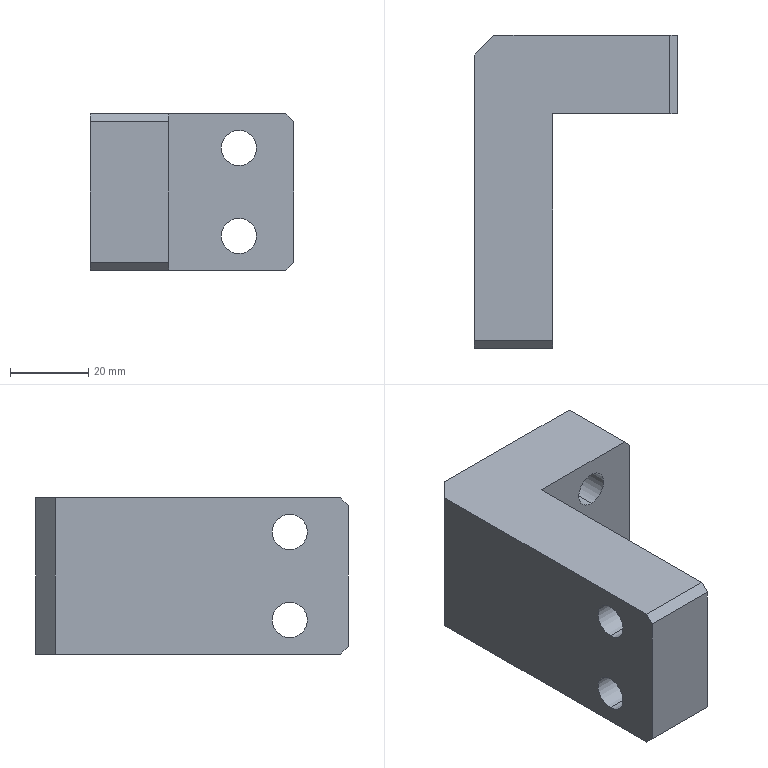Part | SolidWorks | features BaseBody 1 | 1 solid | 33 faces | box 52 x 80 x 40 mm | volume 79960 mm3 | plane 17 | cylinder 16 | commonest cylinder face diameters 9 x8 15 x8
STEP:
#1=CARTESIAN_POINT('',(104.247,1717.,-362.75));
#2=VERTEX_POINT('',#1);
#3=CARTESIAN_POINT('',(104.247,1717.,-353.75));
#4=VERTEX_POINT('',#3);
#5=CARTESIAN_POINT('',(104.247,1717.,-358.25));
#6=DIRECTION('',(-1.,0.,0.));
#7=DIRECTION('',(0.,0.,-1.));
#8=AXIS2_PLACEMENT_3D('',#5,#6,#7);
#9=CIRCLE('',#8,4.5);
#10=EDGE_CURVE('',#2,#4,#9,.T.);
#11=ORIENTED_EDGE('',*,*,#10,.T.);
#12=CARTESIAN_POINT('',(115.647,1717.,-353.75));
#13=VERTEX_POINT('',#12);
#14=CARTESIAN_POINT('',(124.247,1717.,-353.75));
#15=DIRECTION('',(1.,0.,0.));
#16=VECTOR('',#15,1000.);
#17=LINE('',#14,#16);
#18=EDGE_CURVE('',#4,#13,#17,.T.);
#19=ORIENTED_EDGE('',*,*,#18,.T.);
#20=CARTESIAN_POINT('',(115.647,1717.,-362.75));
#21=VERTEX_POINT('',#20);
#22=CARTESIAN_POINT('',(115.647,1717.,-358.25));
#23=DIRECTION('',(-1.,0.,0.));
#24=DIRECTION('',(0.,0.,-1.));
#25=AXIS2_PLACEMENT_3D('',#22,#23,#24);
#26=CIRCLE('',#25,4.5);
#27=EDGE_CURVE('',#21,#13,#26,.T.);
#28=ORIENTED_EDGE('',*,*,#27,.F.);
#29=CARTESIAN_POINT('',(124.247,1717.,-362.75));
#30=DIRECTION('',(1.,0.,0.));
#31=VECTOR('',#30,1000.);
#32=LINE('',#29,#31);
#33=EDGE_CURVE('',#2,#21,#32,.T.);
#34=ORIENTED_EDGE('',*,*,#33,.F.);
#35=EDGE_LOOP('',(#11,#19,#28,#34));
#36=FACE_OUTER_BOUND('',#35,.T.);
#37=CARTESIAN_POINT('',(124.247,1717.,-358.25));
#38=DIRECTION('',(1.,0.,0.));
#39=DIRECTION('',(0.,0.,-1.));
#40=AXIS2_PLACEMENT_3D('',#37,#38,#39);
#41=CYLINDRICAL_SURFACE('',#40,4.5);
#42=ADVANCED_FACE('',(#36),#41,.F.);
#43=CARTESIAN_POINT('',(104.247,1717.,-340.25));
#44=VERTEX_POINT('',#43);
#45=CARTESIAN_POINT('',(104.247,1717.,-331.25));
#46=VERTEX_POINT('',#45);
#47=CARTESIAN_POINT('',(104.247,1717.,-335.75));
#48=DIRECTION('',(-1.,0.,0.));
#49=DIRECTION('',(0.,0.,-1.));
#50=AXIS2_PLACEMENT_3D('',#47,#48,#49);
#51=CIRCLE('',#50,4.5);
#52=EDGE_CURVE('',#44,#46,#51,.T.);
#53=ORIENTED_EDGE('',*,*,#52,.T.);
#54=CARTESIAN_POINT('',(115.647,1717.,-331.25));
#55=VERTEX_POINT('',#54);
#56=CARTESIAN_POINT('',(124.247,1717.,-331.25));
#57=DIRECTION('',(1.,0.,0.));
#58=VECTOR('',#57,1000.);
#59=LINE('',#56,#58);
#60=EDGE_CURVE('',#46,#55,#59,.T.);
#61=ORIENTED_EDGE('',*,*,#60,.T.);
#62=CARTESIAN_POINT('',(115.647,1717.,-340.25));
#63=VERTEX_POINT('',#62);
#64=CARTESIAN_POINT('',(115.647,1717.,-335.75));
#65=DIRECTION('',(-1.,0.,0.));
#66=DIRECTION('',(0.,0.,-1.));
#67=AXIS2_PLACEMENT_3D('',#64,#65,#66);
#68=CIRCLE('',#67,4.5);
#69=EDGE_CURVE('',#63,#55,#68,.T.);
#70=ORIENTED_EDGE('',*,*,#69,.F.);
#71=CARTESIAN_POINT('',(124.247,1717.,-340.25));
#72=DIRECTION('',(1.,0.,0.));
#73=VECTOR('',#72,1000.);
#74=LINE('',#71,#73);
#75=EDGE_CURVE('',#44,#63,#74,.T.);
#76=ORIENTED_EDGE('',*,*,#75,.F.);
#77=EDGE_LOOP('',(#53,#61,#70,#76));
#78=FACE_OUTER_BOUND('',#77,.T.);
#79=CARTESIAN_POINT('',(124.247,1717.,-335.75));
#80=DIRECTION('',(1.,0.,0.));
#81=DIRECTION('',(0.,0.,-1.));
#82=AXIS2_PLACEMENT_3D('',#79,#80,#81);
#83=CYLINDRICAL_SURFACE('',#82,4.5);
#84=ADVANCED_FACE('',(#78),#83,.F.);
#85=CARTESIAN_POINT('',(115.647,1717.,-365.75));
#86=VERTEX_POINT('',#85);
#87=CARTESIAN_POINT('',(115.647,1717.,-350.75));
#88=VERTEX_POINT('',#87);
#89=CARTESIAN_POINT('',(115.647,1717.,-358.25));
#90=DIRECTION('',(-1.,0.,0.));
#91=DIRECTION('',(0.,0.,-1.));
#92=AXIS2_PLACEMENT_3D('',#89,#90,#91);
#93=CIRCLE('',#92,7.5);
#94=EDGE_CURVE('',#86,#88,#93,.T.);
#95=ORIENTED_EDGE('',*,*,#94,.T.);
#96=CARTESIAN_POINT('',(124.247,1717.,-350.75));
#97=VERTEX_POINT('',#96);
#98=CARTESIAN_POINT('',(124.247,1717.,-350.75));
#99=DIRECTION('',(1.,0.,0.));
#100=VECTOR('',#99,1000.);
#101=LINE('',#98,#100);
#102=EDGE_CURVE('',#88,#97,#101,.T.);
#103=ORIENTED_EDGE('',*,*,#102,.T.);
#104=CARTESIAN_POINT('',(124.247,1717.,-365.75));
#105=VERTEX_POINT('',#104);
#106=CARTESIAN_POINT('',(124.247,1717.,-358.25));
#107=DIRECTION('',(-1.,0.,0.));
#108=DIRECTION('',(0.,0.,-1.));
#109=AXIS2_PLACEMENT_3D('',#106,#107,#108);
#110=CIRCLE('',#109,7.5);
#111=EDGE_CURVE('',#105,#97,#110,.T.);
#112=ORIENTED_EDGE('',*,*,#111,.F.);
#113=CARTESIAN_POINT('',(124.247,1717.,-365.75));
#114=DIRECTION('',(1.,0.,0.));
#115=VECTOR('',#114,1000.);
#116=LINE('',#113,#115);
#117=EDGE_CURVE('',#86,#105,#116,.T.);
#118=ORIENTED_EDGE('',*,*,#117,.F.);
#119=EDGE_LOOP('',(#95,#103,#112,#118));
#120=FACE_OUTER_BOUND('',#119,.T.);
#121=CARTESIAN_POINT('',(124.247,1717.,-358.25));
#122=DIRECTION('',(1.,0.,0.));
#123=DIRECTION('',(0.,0.,-1.));
#124=AXIS2_PLACEMENT_3D('',#121,#122,#123);
#125=CYLINDRICAL_SURFACE('',#124,7.5);
#126=ADVANCED_FACE('',(#120),#125,.F.);
#127=CARTESIAN_POINT('',(115.647,1717.,-343.25));
#128=VERTEX_POINT('',#127);
#129=CARTESIAN_POINT('',(115.647,1717.,-328.25));
#130=VERTEX_POINT('',#129);
#131=CARTESIAN_POINT('',(115.647,1717.,-335.75));
#132=DIRECTION('',(-1.,0.,0.));
#133=DIRECTION('',(0.,0.,-1.));
#134=AXIS2_PLACEMENT_3D('',#131,#132,#133);
#135=CIRCLE('',#134,7.5);
#136=EDGE_CURVE('',#128,#130,#135,.T.);
#137=ORIENTED_EDGE('',*,*,#136,.T.);
#138=CARTESIAN_POINT('',(124.247,1717.,-328.25));
#139=VERTEX_POINT('',#138);
#140=CARTESIAN_POINT('',(124.247,1717.,-328.25));
#141=DIRECTION('',(1.,0.,0.));
#142=VECTOR('',#141,1000.);
#143=LINE('',#140,#142);
#144=EDGE_CURVE('',#130,#139,#143,.T.);
#145=ORIENTED_EDGE('',*,*,#144,.T.);
#146=CARTESIAN_POINT('',(124.247,1717.,-343.25));
#147=VERTEX_POINT('',#146);
#148=CARTESIAN_POINT('',(124.247,1717.,-335.75));
#149=DIRECTION('',(-1.,0.,0.));
#150=DIRECTION('',(0.,0.,-1.));
#151=AXIS2_PLACEMENT_3D('',#148,#149,#150);
#152=CIRCLE('',#151,7.5);
#153=EDGE_CURVE('',#147,#139,#152,.T.);
#154=ORIENTED_EDGE('',*,*,#153,.F.);
#155=CARTESIAN_POINT('',(124.247,1717.,-343.25));
#156=DIRECTION('',(1.,0.,0.));
#157=VECTOR('',#156,1000.);
#158=LINE('',#155,#157);
#159=EDGE_CURVE('',#128,#147,#158,.T.);
#160=ORIENTED_EDGE('',*,*,#159,.F.);
#161=EDGE_LOOP('',(#137,#145,#154,#160));
#162=FACE_OUTER_BOUND('',#161,.T.);
#163=CARTESIAN_POINT('',(124.247,1717.,-335.75));
#164=DIRECTION('',(1.,0.,0.));
#165=DIRECTION('',(0.,0.,-1.));
#166=AXIS2_PLACEMENT_3D('',#163,#164,#165);
#167=CYLINDRICAL_SURFACE('',#166,7.5);
#168=ADVANCED_FACE('',(#162),#167,.F.);
#169=CARTESIAN_POINT('',(142.247,1762.,-362.75));
#170=VERTEX_POINT('',#169);
#171=CARTESIAN_POINT('',(142.247,1762.,-353.75));
#172=VERTEX_POINT('',#171);
#173=CARTESIAN_POINT('',(142.247,1762.,-358.25));
#174=DIRECTION('',(0.,1.,0.));
#175=DIRECTION('',(0.,0.,1.));
#176=AXIS2_PLACEMENT_3D('',#173,#174,#175);
#177=CIRCLE('',#176,4.5);
#178=EDGE_CURVE('',#170,#172,#177,.T.);
#179=ORIENTED_EDGE('',*,*,#178,.F.);
#180=CARTESIAN_POINT('',(142.247,1773.4,-362.75));
#181=VERTEX_POINT('',#180);
#182=CARTESIAN_POINT('',(142.247,1782.,-362.75));
#183=DIRECTION('',(0.,1.,0.));
#184=VECTOR('',#183,1000.);
#185=LINE('',#182,#184);
#186=EDGE_CURVE('',#170,#181,#185,.T.);
#187=ORIENTED_EDGE('',*,*,#186,.T.);
#188=CARTESIAN_POINT('',(142.247,1773.4,-353.75));
#189=VERTEX_POINT('',#188);
#190=CARTESIAN_POINT('',(142.247,1773.4,-358.25));
#191=DIRECTION('',(0.,-1.,0.));
#192=DIRECTION('',(0.,0.,1.));
#193=AXIS2_PLACEMENT_3D('',#190,#191,#192);
#194=CIRCLE('',#193,4.5);
#195=EDGE_CURVE('',#189,#181,#194,.T.);
#196=ORIENTED_EDGE('',*,*,#195,.F.);
#197=CARTESIAN_POINT('',(142.247,1782.,-353.75));
#198=DIRECTION('',(0.,1.,0.));
#199=VECTOR('',#198,1000.);
#200=LINE('',#197,#199);
#201=EDGE_CURVE('',#172,#189,#200,.T.);
#202=ORIENTED_EDGE('',*,*,#201,.F.);
#203=EDGE_LOOP('',(#179,#187,#196,#202));
#204=FACE_OUTER_BOUND('',#203,.T.);
#205=CARTESIAN_POINT('',(142.247,1782.,-358.25));
#206=DIRECTION('',(0.,1.,0.));
#207=DIRECTION('',(0.,0.,1.));
#208=AXIS2_PLACEMENT_3D('',#205,#206,#207);
#209=CYLINDRICAL_SURFACE('',#208,4.5);
#210=ADVANCED_FACE('',(#204),#209,.F.);
#211=CARTESIAN_POINT('',(142.247,1762.,-340.25));
#212=VERTEX_POINT('',#211);
#213=CARTESIAN_POINT('',(142.247,1762.,-331.25));
#214=VERTEX_POINT('',#213);
#215=CARTESIAN_POINT('',(142.247,1762.,-335.75));
#216=DIRECTION('',(0.,1.,0.));
#217=DIRECTION('',(0.,0.,1.));
#218=AXIS2_PLACEMENT_3D('',#215,#216,#217);
#219=CIRCLE('',#218,4.5);
#220=EDGE_CURVE('',#212,#214,#219,.T.);
#221=ORIENTED_EDGE('',*,*,#220,.F.);
#222=CARTESIAN_POINT('',(142.247,1773.4,-340.25));
#223=VERTEX_POINT('',#222);
#224=CARTESIAN_POINT('',(142.247,1782.,-340.25));
#225=DIRECTION('',(0.,1.,0.));
#226=VECTOR('',#225,1000.);
#227=LINE('',#224,#226);
#228=EDGE_CURVE('',#212,#223,#227,.T.);
#229=ORIENTED_EDGE('',*,*,#228,.T.);
#230=CARTESIAN_POINT('',(142.247,1773.4,-331.25));
#231=VERTEX_POINT('',#230);
#232=CARTESIAN_POINT('',(142.247,1773.4,-335.75));
#233=DIRECTION('',(0.,-1.,0.));
#234=DIRECTION('',(0.,0.,1.));
#235=AXIS2_PLACEMENT_3D('',#232,#233,#234);
#236=CIRCLE('',#235,4.5);
#237=EDGE_CURVE('',#231,#223,#236,.T.);
#238=ORIENTED_EDGE('',*,*,#237,.F.);
#239=CARTESIAN_POINT('',(142.247,1782.,-331.25));
#240=DIRECTION('',(0.,1.,0.));
#241=VECTOR('',#240,1000.);
#242=LINE('',#239,#241);
#243=EDGE_CURVE('',#214,#231,#242,.T.);
#244=ORIENTED_EDGE('',*,*,#243,.F.);
#245=EDGE_LOOP('',(#221,#229,#238,#244));
#246=FACE_OUTER_BOUND('',#245,.T.);
#247=CARTESIAN_POINT('',(142.247,1782.,-335.75));
#248=DIRECTION('',(0.,1.,0.));
#249=DIRECTION('',(0.,0.,1.));
#250=AXIS2_PLACEMENT_3D('',#247,#248,#249);
#251=CYLINDRICAL_SURFACE('',#250,4.5);
#252=ADVANCED_FACE('',(#246),#251,.F.);
#253=CARTESIAN_POINT('',(142.247,1773.4,-365.75));
#254=VERTEX_POINT('',#253);
#255=CARTESIAN_POINT('',(142.247,1773.4,-350.75));
#256=VERTEX_POINT('',#255);
#257=CARTESIAN_POINT('',(142.247,1773.4,-358.25));
#258=DIRECTION('',(0.,1.,0.));
#259=DIRECTION('',(0.,0.,1.));
#260=AXIS2_PLACEMENT_3D('',#257,#258,#259);
#261=CIRCLE('',#260,7.5);
#262=EDGE_CURVE('',#254,#256,#261,.T.);
#263=ORIENTED_EDGE('',*,*,#262,.F.);
#264=CARTESIAN_POINT('',(142.247,1782.,-365.75));
#265=VERTEX_POINT('',#264);
#266=CARTESIAN_POINT('',(142.247,1782.,-365.75));
#267=DIRECTION('',(0.,1.,0.));
#268=VECTOR('',#267,1000.);
#269=LINE('',#266,#268);
#270=EDGE_CURVE('',#254,#265,#269,.T.);
#271=ORIENTED_EDGE('',*,*,#270,.T.);
#272=CARTESIAN_POINT('',(142.247,1782.,-350.75));
#273=VERTEX_POINT('',#272);
#274=CARTESIAN_POINT('',(142.247,1782.,-358.25));
#275=DIRECTION('',(0.,1.,0.));
#276=DIRECTION('',(0.,0.,1.));
#277=AXIS2_PLACEMENT_3D('',#274,#275,#276);
#278=CIRCLE('',#277,7.5);
#279=EDGE_CURVE('',#265,#273,#278,.T.);
#280=ORIENTED_EDGE('',*,*,#279,.T.);
#281=CARTESIAN_POINT('',(142.247,1782.,-350.75));
#282=DIRECTION('',(0.,1.,0.));
#283=VECTOR('',#282,1000.);
#284=LINE('',#281,#283);
#285=EDGE_CURVE('',#256,#273,#284,.T.);
#286=ORIENTED_EDGE('',*,*,#285,.F.);
#287=EDGE_LOOP('',(#263,#271,#280,#286));
#288=FACE_OUTER_BOUND('',#287,.T.);
#289=CARTESIAN_POINT('',(142.247,1782.,-358.25));
#290=DIRECTION('',(0.,1.,0.));
#291=DIRECTION('',(0.,0.,1.));
#292=AXIS2_PLACEMENT_3D('',#289,#290,#291);
#293=CYLINDRICAL_SURFACE('',#292,7.5);
#294=ADVANCED_FACE('',(#288),#293,.F.);
#295=CARTESIAN_POINT('',(142.247,1773.4,-343.25));
#296=VERTEX_POINT('',#295);
#297=CARTESIAN_POINT('',(142.247,1773.4,-328.25));
#298=VERTEX_POINT('',#297);
#299=CARTESIAN_POINT('',(142.247,1773.4,-335.75));
#300=DIRECTION('',(0.,1.,0.));
#301=DIRECTION('',(0.,0.,1.));
#302=AXIS2_PLACEMENT_3D('',#299,#300,#301);
#303=CIRCLE('',#302,7.5);
#304=EDGE_CURVE('',#296,#298,#303,.T.);
#305=ORIENTED_EDGE('',*,*,#304,.F.);
#306=CARTESIAN_POINT('',(142.247,1782.,-343.25));
#307=VERTEX_POINT('',#306);
#308=CARTESIAN_POINT('',(142.247,1782.,-343.25));
#309=DIRECTION('',(0.,1.,0.));
#310=VECTOR('',#309,1000.);
#311=LINE('',#308,#310);
#312=EDGE_CURVE('',#296,#307,#311,.T.);
#313=ORIENTED_EDGE('',*,*,#312,.T.);
#314=CARTESIAN_POINT('',(142.247,1782.,-328.25));
#315=VERTEX_POINT('',#314);
#316=CARTESIAN_POINT('',(142.247,1782.,-335.75));
#317=DIRECTION('',(0.,1.,0.));
#318=DIRECTION('',(0.,0.,1.));
#319=AXIS2_PLACEMENT_3D('',#316,#317,#318);
#320=CIRCLE('',#319,7.5);
#321=EDGE_CURVE('',#307,#315,#320,.T.);
#322=ORIENTED_EDGE('',*,*,#321,.T.);
#323=CARTESIAN_POINT('',(142.247,1782.,-328.25));
#324=DIRECTION('',(0.,1.,0.));
#325=VECTOR('',#324,1000.);
#326=LINE('',#323,#325);
#327=EDGE_CURVE('',#298,#315,#326,.T.);
#328=ORIENTED_EDGE('',*,*,#327,.F.);
#329=EDGE_LOOP('',(#305,#313,#322,#328));
#330=FACE_OUTER_BOUND('',#329,.T.);
#331=CARTESIAN_POINT('',(142.247,1782.,-335.75));
#332=DIRECTION('',(0.,1.,0.));
#333=DIRECTION('',(0.,0.,1.));
#334=AXIS2_PLACEMENT_3D('',#331,#332,#333);
#335=CYLINDRICAL_SURFACE('',#334,7.5);
#336=ADVANCED_FACE('',(#330),#335,.F.);
#337=ORIENTED_EDGE('',*,*,#10,.F.);
#338=CARTESIAN_POINT('',(104.247,1717.,-358.25));
#339=DIRECTION('',(-1.,0.,0.));
#340=DIRECTION('',(0.,0.,-1.));
#341=AXIS2_PLACEMENT_3D('',#338,#339,#340);
#342=CIRCLE('',#341,4.5);
#343=EDGE_CURVE('',#4,#2,#342,.T.);
#344=ORIENTED_EDGE('',*,*,#343,.F.);
#345=EDGE_LOOP('',(#337,#344));
#346=FACE_BOUND('',#345,.T.);
#347=ORIENTED_EDGE('',*,*,#52,.F.);
#348=CARTESIAN_POINT('',(104.247,1717.,-335.75));
#349=DIRECTION('',(-1.,0.,0.));
#350=DIRECTION('',(0.,0.,-1.));
#351=AXIS2_PLACEMENT_3D('',#348,#349,#350);
#352=CIRCLE('',#351,4.5);
#353=EDGE_CURVE('',#46,#44,#352,.T.);
#354=ORIENTED_EDGE('',*,*,#353,.F.);
#355=EDGE_LOOP('',(#347,#354));
#356=FACE_BOUND('',#355,.T.);
#357=CARTESIAN_POINT('',(104.247,1777.,-327.));
#358=VERTEX_POINT('',#357);
#359=CARTESIAN_POINT('',(104.247,1704.,-327.));
#360=VERTEX_POINT('',#359);
#361=CARTESIAN_POINT('',(104.247,1702.,-327.));
#362=DIRECTION('',(0.,-1.,0.));
#363=VECTOR('',#362,1000.);
#364=LINE('',#361,#363);
#365=EDGE_CURVE('',#358,#360,#364,.T.);
#366=ORIENTED_EDGE('',*,*,#365,.F.);
#367=CARTESIAN_POINT('',(104.247,1777.,-367.));
#368=VERTEX_POINT('',#367);
#369=CARTESIAN_POINT('',(104.247,1777.,-367.));
#370=DIRECTION('',(0.,0.,1.));
#371=VECTOR('',#370,1000.);
#372=LINE('',#369,#371);
#373=EDGE_CURVE('',#368,#358,#372,.T.);
#374=ORIENTED_EDGE('',*,*,#373,.F.);
#375=CARTESIAN_POINT('',(104.247,1704.,-367.));
#376=VERTEX_POINT('',#375);
#377=CARTESIAN_POINT('',(104.247,1702.,-367.));
#378=DIRECTION('',(0.,1.,0.));
#379=VECTOR('',#378,1000.);
#380=LINE('',#377,#379);
#381=EDGE_CURVE('',#376,#368,#380,.T.);
#382=ORIENTED_EDGE('',*,*,#381,.F.);
#383=CARTESIAN_POINT('',(104.247,1702.,-365.));
#384=VERTEX_POINT('',#383);
#385=CARTESIAN_POINT('',(104.247,1702.,-365.));
#386=DIRECTION('',(0.,0.7071,-0.7071));
#387=VECTOR('',#386,1000.);
#388=LINE('',#385,#387);
#389=EDGE_CURVE('',#384,#376,#388,.T.);
#390=ORIENTED_EDGE('',*,*,#389,.F.);
#391=CARTESIAN_POINT('',(104.247,1702.,-329.));
#392=VERTEX_POINT('',#391);
#393=CARTESIAN_POINT('',(104.247,1702.,-367.));
#394=DIRECTION('',(0.,0.,-1.));
#395=VECTOR('',#394,1000.);
#396=LINE('',#393,#395);
#397=EDGE_CURVE('',#392,#384,#396,.T.);
#398=ORIENTED_EDGE('',*,*,#397,.F.);
#399=CARTESIAN_POINT('',(104.247,1704.,-327.));
#400=DIRECTION('',(0.,-0.7071,-0.7071));
#401=VECTOR('',#400,1000.);
#402=LINE('',#399,#401);
#403=EDGE_CURVE('',#360,#392,#402,.T.);
#404=ORIENTED_EDGE('',*,*,#403,.F.);
#405=EDGE_LOOP('',(#366,#374,#382,#390,#398,#404));
#406=FACE_OUTER_BOUND('',#405,.T.);
#407=CARTESIAN_POINT('',(104.247,1702.,-367.));
#408=DIRECTION('',(1.,0.,0.));
#409=DIRECTION('',(0.,0.,-1.));
#410=AXIS2_PLACEMENT_3D('',#407,#408,#409);
#411=PLANE('',#410);
#412=ADVANCED_FACE('',(#346,#356,#406),#411,.F.);
#413=ORIENTED_EDGE('',*,*,#18,.F.);
#414=ORIENTED_EDGE('',*,*,#343,.T.);
#415=ORIENTED_EDGE('',*,*,#33,.T.);
#416=CARTESIAN_POINT('',(115.647,1717.,-358.25));
#417=DIRECTION('',(-1.,0.,0.));
#418=DIRECTION('',(0.,0.,-1.));
#419=AXIS2_PLACEMENT_3D('',#416,#417,#418);
#420=CIRCLE('',#419,4.5);
#421=EDGE_CURVE('',#13,#21,#420,.T.);
#422=ORIENTED_EDGE('',*,*,#421,.F.);
#423=EDGE_LOOP('',(#413,#414,#415,#422));
#424=FACE_OUTER_BOUND('',#423,.T.);
#425=CARTESIAN_POINT('',(124.247,1717.,-358.25));
#426=DIRECTION('',(1.,0.,0.));
#427=DIRECTION('',(0.,0.,-1.));
#428=AXIS2_PLACEMENT_3D('',#425,#426,#427);
#429=CYLINDRICAL_SURFACE('',#428,4.5);
#430=ADVANCED_FACE('',(#424),#429,.F.);
#431=ORIENTED_EDGE('',*,*,#60,.F.);
#432=ORIENTED_EDGE('',*,*,#353,.T.);
#433=ORIENTED_EDGE('',*,*,#75,.T.);
#434=CARTESIAN_POINT('',(115.647,1717.,-335.75));
#435=DIRECTION('',(-1.,0.,0.));
#436=DIRECTION('',(0.,0.,-1.));
#437=AXIS2_PLACEMENT_3D('',#434,#435,#436);
#438=CIRCLE('',#437,4.5);
#439=EDGE_CURVE('',#55,#63,#438,.T.);
#440=ORIENTED_EDGE('',*,*,#439,.F.);
#441=EDGE_LOOP('',(#431,#432,#433,#440));
#442=FACE_OUTER_BOUND('',#441,.T.);
#443=CARTESIAN_POINT('',(124.247,1717.,-335.75));
#444=DIRECTION('',(1.,0.,0.));
#445=DIRECTION('',(0.,0.,-1.));
#446=AXIS2_PLACEMENT_3D('',#443,#444,#445);
#447=CYLINDRICAL_SURFACE('',#446,4.5);
#448=ADVANCED_FACE('',(#442),#447,.F.);
#449=ORIENTED_EDGE('',*,*,#403,.T.);
#450=CARTESIAN_POINT('',(124.247,1702.,-329.));
#451=VERTEX_POINT('',#450);
#452=CARTESIAN_POINT('',(104.247,1702.,-329.));
#453=DIRECTION('',(-1.,0.,0.));
#454=VECTOR('',#453,1000.);
#455=LINE('',#452,#454);
#456=EDGE_CURVE('',#451,#392,#455,.T.);
#457=ORIENTED_EDGE('',*,*,#456,.F.);
#458=CARTESIAN_POINT('',(124.247,1704.,-327.));
#459=VERTEX_POINT('',#458);
#460=CARTESIAN_POINT('',(124.247,1702.,-329.));
#461=DIRECTION('',(0.,-0.7071,-0.7071));
#462=VECTOR('',#461,1000.);
#463=LINE('',#460,#462);
#464=EDGE_CURVE('',#459,#451,#463,.T.);
#465=ORIENTED_EDGE('',*,*,#464,.F.);
#466=CARTESIAN_POINT('',(104.247,1704.,-327.));
#467=DIRECTION('',(1.,0.,0.));
#468=VECTOR('',#467,1000.);
#469=LINE('',#466,#468);
#470=EDGE_CURVE('',#360,#459,#469,.T.);
#471=ORIENTED_EDGE('',*,*,#470,.F.);
#472=EDGE_LOOP('',(#449,#457,#465,#471));
#473=FACE_OUTER_BOUND('',#472,.T.);
#474=CARTESIAN_POINT('',(104.247,1702.,-329.));
#475=DIRECTION('',(0.,0.7071,-0.7071));
#476=DIRECTION('',(0.,0.7071,0.7071));
#477=AXIS2_PLACEMENT_3D('',#474,#475,#476);
#478=PLANE('',#477);
#479=ADVANCED_FACE('',(#473),#478,.F.);
#480=CARTESIAN_POINT('',(124.247,1762.,-327.));
#481=VERTEX_POINT('',#480);
#482=CARTESIAN_POINT('',(124.247,1702.,-327.));
#483=DIRECTION('',(0.,-1.,0.));
#484=VECTOR('',#483,1000.);
#485=LINE('',#482,#484);
#486=EDGE_CURVE('',#481,#459,#485,.T.);
#487=ORIENTED_EDGE('',*,*,#486,.F.);
#488=CARTESIAN_POINT('',(154.247,1762.,-327.));
#489=VERTEX_POINT('',#488);
#490=CARTESIAN_POINT('',(104.247,1762.,-327.));
#491=DIRECTION('',(-1.,0.,0.));
#492=VECTOR('',#491,1000.);
#493=LINE('',#490,#492);
#494=EDGE_CURVE('',#489,#481,#493,.T.);
#495=ORIENTED_EDGE('',*,*,#494,.F.);
#496=CARTESIAN_POINT('',(154.247,1782.,-327.));
#497=VERTEX_POINT('',#496);
#498=CARTESIAN_POINT('',(154.247,1702.,-327.));
#499=DIRECTION('',(0.,-1.,0.));
#500=VECTOR('',#499,1000.);
#501=LINE('',#498,#500);
#502=EDGE_CURVE('',#497,#489,#501,.T.);
#503=ORIENTED_EDGE('',*,*,#502,.F.);
#504=CARTESIAN_POINT('',(109.247,1782.,-327.));
#505=VERTEX_POINT('',#504);
#506=CARTESIAN_POINT('',(104.247,1782.,-327.));
#507=DIRECTION('',(1.,0.,0.));
#508=VECTOR('',#507,1000.);
#509=LINE('',#506,#508);
#510=EDGE_CURVE('',#505,#497,#509,.T.);
#511=ORIENTED_EDGE('',*,*,#510,.F.);
#512=CARTESIAN_POINT('',(104.247,1777.,-327.));
#513=DIRECTION('',(0.7071,0.7071,0.));
#514=VECTOR('',#513,1000.);
#515=LINE('',#512,#514);
#516=EDGE_CURVE('',#358,#505,#515,.T.);
#517=ORIENTED_EDGE('',*,*,#516,.F.);
#518=ORIENTED_EDGE('',*,*,#365,.T.);
#519=ORIENTED_EDGE('',*,*,#470,.T.);
#520=EDGE_LOOP('',(#487,#495,#503,#511,#517,#518,#519));
#521=FACE_OUTER_BOUND('',#520,.T.);
#522=CARTESIAN_POINT('',(104.247,1702.,-327.));
#523=DIRECTION('',(0.,0.,-1.));
#524=DIRECTION('',(-1.,0.,0.));
#525=AXIS2_PLACEMENT_3D('',#522,#523,#524);
#526=PLANE('',#525);
#527=ADVANCED_FACE('',(#521),#526,.F.);
#528=ORIENTED_EDGE('',*,*,#516,.T.);
#529=CARTESIAN_POINT('',(109.247,1782.,-367.));
#530=VERTEX_POINT('',#529);
#531=CARTESIAN_POINT('',(109.247,1782.,-367.));
#532=DIRECTION('',(0.,0.,1.));
#533=VECTOR('',#532,1000.);
#534=LINE('',#531,#533);
#535=EDGE_CURVE('',#530,#505,#534,.T.);
#536=ORIENTED_EDGE('',*,*,#535,.F.);
#537=CARTESIAN_POINT('',(109.247,1782.,-367.));
#538=DIRECTION('',(0.7071,0.7071,0.));
#539=VECTOR('',#538,1000.);
#540=LINE('',#537,#539);
#541=EDGE_CURVE('',#368,#530,#540,.T.);
#542=ORIENTED_EDGE('',*,*,#541,.F.);
#543=ORIENTED_EDGE('',*,*,#373,.T.);
#544=EDGE_LOOP('',(#528,#536,#542,#543));
#545=FACE_OUTER_BOUND('',#544,.T.);
#546=CARTESIAN_POINT('',(109.247,1782.,-367.));
#547=DIRECTION('',(0.7071,-0.7071,0.));
#548=DIRECTION('',(0.7071,0.7071,0.));
#549=AXIS2_PLACEMENT_3D('',#546,#547,#548);
#550=PLANE('',#549);
#551=ADVANCED_FACE('',(#545),#550,.F.);
#552=CARTESIAN_POINT('',(154.247,1762.,-367.));
#553=VERTEX_POINT('',#552);
#554=CARTESIAN_POINT('',(124.247,1762.,-367.));
#555=VERTEX_POINT('',#554);
#556=CARTESIAN_POINT('',(104.247,1762.,-367.));
#557=DIRECTION('',(-1.,0.,0.));
#558=VECTOR('',#557,1000.);
#559=LINE('',#556,#558);
#560=EDGE_CURVE('',#553,#555,#559,.T.);
#561=ORIENTED_EDGE('',*,*,#560,.T.);
#562=CARTESIAN_POINT('',(124.247,1704.,-367.));
#563=VERTEX_POINT('',#562);
#564=CARTESIAN_POINT('',(124.247,1702.,-367.));
#565=DIRECTION('',(0.,-1.,0.));
#566=VECTOR('',#565,1000.);
#567=LINE('',#564,#566);
#568=EDGE_CURVE('',#555,#563,#567,.T.);
#569=ORIENTED_EDGE('',*,*,#568,.T.);
#570=CARTESIAN_POINT('',(104.247,1704.,-367.));
#571=DIRECTION('',(-1.,0.,0.));
#572=VECTOR('',#571,1000.);
#573=LINE('',#570,#572);
#574=EDGE_CURVE('',#563,#376,#573,.T.);
#575=ORIENTED_EDGE('',*,*,#574,.T.);
#576=ORIENTED_EDGE('',*,*,#381,.T.);
#577=ORIENTED_EDGE('',*,*,#541,.T.);
#578=CARTESIAN_POINT('',(154.247,1782.,-367.));
#579=VERTEX_POINT('',#578);
#580=CARTESIAN_POINT('',(104.247,1782.,-367.));
#581=DIRECTION('',(1.,0.,0.));
#582=VECTOR('',#581,1000.);
#583=LINE('',#580,#582);
#584=EDGE_CURVE('',#530,#579,#583,.T.);
#585=ORIENTED_EDGE('',*,*,#584,.T.);
#586=CARTESIAN_POINT('',(154.247,1702.,-367.));
#587=DIRECTION('',(0.,-1.,0.));
#588=VECTOR('',#587,1000.);
#589=LINE('',#586,#588);
#590=EDGE_CURVE('',#579,#553,#589,.T.);
#591=ORIENTED_EDGE('',*,*,#590,.T.);
#592=EDGE_LOOP('',(#561,#569,#575,#576,#577,#585,#591));
#593=FACE_OUTER_BOUND('',#592,.T.);
#594=CARTESIAN_POINT('',(104.247,1702.,-367.));
#595=DIRECTION('',(0.,0.,-1.));
#596=DIRECTION('',(-1.,0.,0.));
#597=AXIS2_PLACEMENT_3D('',#594,#595,#596);
#598=PLANE('',#597);
#599=ADVANCED_FACE('',(#593),#598,.T.);
#600=ORIENTED_EDGE('',*,*,#574,.F.);
#601=CARTESIAN_POINT('',(124.247,1702.,-365.));
#602=VERTEX_POINT('',#601);
#603=CARTESIAN_POINT('',(124.247,1704.,-367.));
#604=DIRECTION('',(0.,-0.7071,0.7071));
#605=VECTOR('',#604,1000.);
#606=LINE('',#603,#605);
#607=EDGE_CURVE('',#563,#602,#606,.T.);
#608=ORIENTED_EDGE('',*,*,#607,.T.);
#609=CARTESIAN_POINT('',(104.247,1702.,-365.));
#610=DIRECTION('',(-1.,0.,0.));
#611=VECTOR('',#610,1000.);
#612=LINE('',#609,#611);
#613=EDGE_CURVE('',#602,#384,#612,.T.);
#614=ORIENTED_EDGE('',*,*,#613,.T.);
#615=ORIENTED_EDGE('',*,*,#389,.T.);
#616=EDGE_LOOP('',(#600,#608,#614,#615));
#617=FACE_OUTER_BOUND('',#616,.T.);
#618=CARTESIAN_POINT('',(104.247,1704.,-367.));
#619=DIRECTION('',(0.,-0.7071,-0.7071));
#620=DIRECTION('',(0.,0.7071,-0.7071));
#621=AXIS2_PLACEMENT_3D('',#618,#619,#620);
#622=PLANE('',#621);
#623=ADVANCED_FACE('',(#617),#622,.T.);
#624=ORIENTED_EDGE('',*,*,#397,.T.);
#625=ORIENTED_EDGE('',*,*,#613,.F.);
#626=CARTESIAN_POINT('',(124.247,1702.,-367.));
#627=DIRECTION('',(0.,0.,-1.));
#628=VECTOR('',#627,1000.);
#629=LINE('',#626,#628);
#630=EDGE_CURVE('',#451,#602,#629,.T.);
#631=ORIENTED_EDGE('',*,*,#630,.F.);
#632=ORIENTED_EDGE('',*,*,#456,.T.);
#633=EDGE_LOOP('',(#624,#625,#631,#632));
#634=FACE_OUTER_BOUND('',#633,.T.);
#635=CARTESIAN_POINT('',(104.247,1702.,-367.));
#636=DIRECTION('',(0.,1.,0.));
#637=DIRECTION('',(0.,0.,1.));
#638=AXIS2_PLACEMENT_3D('',#635,#636,#637);
#639=PLANE('',#638);
#640=ADVANCED_FACE('',(#634),#639,.F.);
#641=ORIENTED_EDGE('',*,*,#27,.T.);
#642=ORIENTED_EDGE('',*,*,#421,.T.);
#643=EDGE_LOOP('',(#641,#642));
#644=FACE_BOUND('',#643,.T.);
#645=ORIENTED_EDGE('',*,*,#94,.F.);
#646=CARTESIAN_POINT('',(115.647,1717.,-358.25));
#647=DIRECTION('',(-1.,0.,0.));
#648=DIRECTION('',(0.,0.,-1.));
#649=AXIS2_PLACEMENT_3D('',#646,#647,#648);
#650=CIRCLE('',#649,7.5);
#651=EDGE_CURVE('',#88,#86,#650,.T.);
#652=ORIENTED_EDGE('',*,*,#651,.F.);
#653=EDGE_LOOP('',(#645,#652));
#654=FACE_OUTER_BOUND('',#653,.T.);
#655=CARTESIAN_POINT('',(115.647,1712.5,-358.25));
#656=DIRECTION('',(-1.,0.,0.));
#657=DIRECTION('',(0.,0.,1.));
#658=AXIS2_PLACEMENT_3D('',#655,#656,#657);
#659=PLANE('',#658);
#660=ADVANCED_FACE('',(#644,#654),#659,.F.);
#661=ORIENTED_EDGE('',*,*,#69,.T.);
#662=ORIENTED_EDGE('',*,*,#439,.T.);
#663=EDGE_LOOP('',(#661,#662));
#664=FACE_BOUND('',#663,.T.);
#665=ORIENTED_EDGE('',*,*,#136,.F.);
#666=CARTESIAN_POINT('',(115.647,1717.,-335.75));
#667=DIRECTION('',(-1.,0.,0.));
#668=DIRECTION('',(0.,0.,-1.));
#669=AXIS2_PLACEMENT_3D('',#666,#667,#668);
#670=CIRCLE('',#669,7.5);
#671=EDGE_CURVE('',#130,#128,#670,.T.);
#672=ORIENTED_EDGE('',*,*,#671,.F.);
#673=EDGE_LOOP('',(#665,#672));
#674=FACE_OUTER_BOUND('',#673,.T.);
#675=CARTESIAN_POINT('',(115.647,1712.5,-335.75));
#676=DIRECTION('',(-1.,0.,0.));
#677=DIRECTION('',(0.,0.,1.));
#678=AXIS2_PLACEMENT_3D('',#675,#676,#677);
#679=PLANE('',#678);
#680=ADVANCED_FACE('',(#664,#674),#679,.F.);
#681=ORIENTED_EDGE('',*,*,#111,.T.);
#682=CARTESIAN_POINT('',(124.247,1717.,-358.25));
#683=DIRECTION('',(-1.,0.,0.));
#684=DIRECTION('',(0.,0.,-1.));
#685=AXIS2_PLACEMENT_3D('',#682,#683,#684);
#686=CIRCLE('',#685,7.5);
#687=EDGE_CURVE('',#97,#105,#686,.T.);
#688=ORIENTED_EDGE('',*,*,#687,.T.);
#689=EDGE_LOOP('',(#681,#688));
#690=FACE_BOUND('',#689,.T.);
#691=ORIENTED_EDGE('',*,*,#153,.T.);
#692=CARTESIAN_POINT('',(124.247,1717.,-335.75));
#693=DIRECTION('',(-1.,0.,0.));
#694=DIRECTION('',(0.,0.,-1.));
#695=AXIS2_PLACEMENT_3D('',#692,#693,#694);
#696=CIRCLE('',#695,7.5);
#697=EDGE_CURVE('',#139,#147,#696,.T.);
#698=ORIENTED_EDGE('',*,*,#697,.T.);
#699=EDGE_LOOP('',(#691,#698));
#700=FACE_BOUND('',#699,.T.);
#701=CARTESIAN_POINT('',(124.247,1762.,-236.645));
#702=DIRECTION('',(0.,0.,1.));
#703=VECTOR('',#702,1000.);
#704=LINE('',#701,#703);
#705=EDGE_CURVE('',#555,#481,#704,.T.);
#706=ORIENTED_EDGE('',*,*,#705,.T.);
#707=ORIENTED_EDGE('',*,*,#486,.T.);
#708=ORIENTED_EDGE('',*,*,#464,.T.);
#709=ORIENTED_EDGE('',*,*,#630,.T.);
#710=ORIENTED_EDGE('',*,*,#607,.F.);
#711=ORIENTED_EDGE('',*,*,#568,.F.);
#712=EDGE_LOOP('',(#706,#707,#708,#709,#710,#711));
#713=FACE_OUTER_BOUND('',#712,.T.);
#714=CARTESIAN_POINT('',(124.247,1702.,-236.645));
#715=DIRECTION('',(1.,0.,0.));
#716=DIRECTION('',(0.,0.,-1.));
#717=AXIS2_PLACEMENT_3D('',#714,#715,#716);
#718=PLANE('',#717);
#719=ADVANCED_FACE('',(#690,#700,#713),#718,.T.);
#720=CARTESIAN_POINT('',(142.247,1762.,-358.25));
#721=DIRECTION('',(0.,1.,0.));
#722=DIRECTION('',(0.,0.,1.));
#723=AXIS2_PLACEMENT_3D('',#720,#721,#722);
#724=CIRCLE('',#723,4.5);
#725=EDGE_CURVE('',#172,#170,#724,.T.);
#726=ORIENTED_EDGE('',*,*,#725,.T.);
#727=ORIENTED_EDGE('',*,*,#178,.T.);
#728=EDGE_LOOP('',(#726,#727));
#729=FACE_BOUND('',#728,.T.);
#730=CARTESIAN_POINT('',(142.247,1762.,-335.75));
#731=DIRECTION('',(0.,1.,0.));
#732=DIRECTION('',(0.,0.,1.));
#733=AXIS2_PLACEMENT_3D('',#730,#731,#732);
#734=CIRCLE('',#733,4.5);
#735=EDGE_CURVE('',#214,#212,#734,.T.);
#736=ORIENTED_EDGE('',*,*,#735,.T.);
#737=ORIENTED_EDGE('',*,*,#220,.T.);
#738=EDGE_LOOP('',(#736,#737));
#739=FACE_BOUND('',#738,.T.);
#740=CARTESIAN_POINT('',(156.247,1762.,-365.));
#741=VERTEX_POINT('',#740);
#742=CARTESIAN_POINT('',(154.247,1762.,-367.));
#743=DIRECTION('',(0.7071,0.,0.7071));
#744=VECTOR('',#743,1000.);
#745=LINE('',#742,#744);
#746=EDGE_CURVE('',#553,#741,#745,.T.);
#747=ORIENTED_EDGE('',*,*,#746,.T.);
#748=CARTESIAN_POINT('',(156.247,1762.,-329.));
#749=VERTEX_POINT('',#748);
#750=CARTESIAN_POINT('',(156.247,1762.,-236.645));
#751=DIRECTION('',(0.,0.,1.));
#752=VECTOR('',#751,1000.);
#753=LINE('',#750,#752);
#754=EDGE_CURVE('',#741,#749,#753,.T.);
#755=ORIENTED_EDGE('',*,*,#754,.T.);
#756=CARTESIAN_POINT('',(156.247,1762.,-329.));
#757=DIRECTION('',(-0.7071,0.,0.7071));
#758=VECTOR('',#757,1000.);
#759=LINE('',#756,#758);
#760=EDGE_CURVE('',#749,#489,#759,.T.);
#761=ORIENTED_EDGE('',*,*,#760,.T.);
#762=ORIENTED_EDGE('',*,*,#494,.T.);
#763=ORIENTED_EDGE('',*,*,#705,.F.);
#764=ORIENTED_EDGE('',*,*,#560,.F.);
#765=EDGE_LOOP('',(#747,#755,#761,#762,#763,#764));
#766=FACE_OUTER_BOUND('',#765,.T.);
#767=CARTESIAN_POINT('',(124.247,1762.,-236.645));
#768=DIRECTION('',(0.,-1.,0.));
#769=DIRECTION('',(0.,0.,-1.));
#770=AXIS2_PLACEMENT_3D('',#767,#768,#769);
#771=PLANE('',#770);
#772=ADVANCED_FACE('',(#729,#739,#766),#771,.T.);
#773=ORIENTED_EDGE('',*,*,#502,.T.);
#774=ORIENTED_EDGE('',*,*,#760,.F.);
#775=CARTESIAN_POINT('',(156.247,1782.,-329.));
#776=VERTEX_POINT('',#775);
#777=CARTESIAN_POINT('',(156.247,1702.,-329.));
#778=DIRECTION('',(0.,1.,0.));
#779=VECTOR('',#778,1000.);
#780=LINE('',#777,#779);
#781=EDGE_CURVE('',#749,#776,#780,.T.);
#782=ORIENTED_EDGE('',*,*,#781,.T.);
#783=CARTESIAN_POINT('',(154.247,1782.,-327.));
#784=DIRECTION('',(-0.7071,0.,0.7071));
#785=VECTOR('',#784,1000.);
#786=LINE('',#783,#785);
#787=EDGE_CURVE('',#776,#497,#786,.T.);
#788=ORIENTED_EDGE('',*,*,#787,.T.);
#789=EDGE_LOOP('',(#773,#774,#782,#788));
#790=FACE_OUTER_BOUND('',#789,.T.);
#791=CARTESIAN_POINT('',(154.247,1702.,-327.));
#792=DIRECTION('',(0.7071,0.,0.7071));
#793=DIRECTION('',(0.7071,0.,-0.7071));
#794=AXIS2_PLACEMENT_3D('',#791,#792,#793);
#795=PLANE('',#794);
#796=ADVANCED_FACE('',(#790),#795,.T.);
#797=CARTESIAN_POINT('',(142.247,1782.,-358.25));
#798=DIRECTION('',(0.,1.,0.));
#799=DIRECTION('',(0.,0.,1.));
#800=AXIS2_PLACEMENT_3D('',#797,#798,#799);
#801=CIRCLE('',#800,7.5);
#802=EDGE_CURVE('',#273,#265,#801,.T.);
#803=ORIENTED_EDGE('',*,*,#802,.F.);
#804=ORIENTED_EDGE('',*,*,#279,.F.);
#805=EDGE_LOOP('',(#803,#804));
#806=FACE_BOUND('',#805,.T.);
#807=CARTESIAN_POINT('',(142.247,1782.,-335.75));
#808=DIRECTION('',(0.,1.,0.));
#809=DIRECTION('',(0.,0.,1.));
#810=AXIS2_PLACEMENT_3D('',#807,#808,#809);
#811=CIRCLE('',#810,7.5);
#812=EDGE_CURVE('',#315,#307,#811,.T.);
#813=ORIENTED_EDGE('',*,*,#812,.F.);
#814=ORIENTED_EDGE('',*,*,#321,.F.);
#815=EDGE_LOOP('',(#813,#814));
#816=FACE_BOUND('',#815,.T.);
#817=CARTESIAN_POINT('',(156.247,1782.,-365.));
#818=VERTEX_POINT('',#817);
#819=CARTESIAN_POINT('',(156.247,1782.,-367.));
#820=DIRECTION('',(0.,0.,1.));
#821=VECTOR('',#820,1000.);
#822=LINE('',#819,#821);
#823=EDGE_CURVE('',#818,#776,#822,.T.);
#824=ORIENTED_EDGE('',*,*,#823,.F.);
#825=CARTESIAN_POINT('',(154.247,1782.,-367.));
#826=DIRECTION('',(0.7071,0.,0.7071));
#827=VECTOR('',#826,1000.);
#828=LINE('',#825,#827);
#829=EDGE_CURVE('',#579,#818,#828,.T.);
#830=ORIENTED_EDGE('',*,*,#829,.F.);
#831=ORIENTED_EDGE('',*,*,#584,.F.);
#832=ORIENTED_EDGE('',*,*,#535,.T.);
#833=ORIENTED_EDGE('',*,*,#510,.T.);
#834=ORIENTED_EDGE('',*,*,#787,.F.);
#835=EDGE_LOOP('',(#824,#830,#831,#832,#833,#834));
#836=FACE_OUTER_BOUND('',#835,.T.);
#837=CARTESIAN_POINT('',(104.247,1782.,-367.));
#838=DIRECTION('',(0.,-1.,0.));
#839=DIRECTION('',(0.,0.,-1.));
#840=AXIS2_PLACEMENT_3D('',#837,#838,#839);
#841=PLANE('',#840);
#842=ADVANCED_FACE('',(#806,#816,#836),#841,.F.);
#843=ORIENTED_EDGE('',*,*,#746,.F.);
#844=ORIENTED_EDGE('',*,*,#590,.F.);
#845=ORIENTED_EDGE('',*,*,#829,.T.);
#846=CARTESIAN_POINT('',(156.247,1702.,-365.));
#847=DIRECTION('',(0.,1.,0.));
#848=VECTOR('',#847,1000.);
#849=LINE('',#846,#848);
#850=EDGE_CURVE('',#741,#818,#849,.T.);
#851=ORIENTED_EDGE('',*,*,#850,.F.);
#852=EDGE_LOOP('',(#843,#844,#845,#851));
#853=FACE_OUTER_BOUND('',#852,.T.);
#854=CARTESIAN_POINT('',(154.247,1702.,-367.));
#855=DIRECTION('',(-0.7071,0.,0.7071));
#856=DIRECTION('',(0.7071,0.,0.7071));
#857=AXIS2_PLACEMENT_3D('',#854,#855,#856);
#858=PLANE('',#857);
#859=ADVANCED_FACE('',(#853),#858,.F.);
#860=ORIENTED_EDGE('',*,*,#102,.F.);
#861=ORIENTED_EDGE('',*,*,#651,.T.);
#862=ORIENTED_EDGE('',*,*,#117,.T.);
#863=ORIENTED_EDGE('',*,*,#687,.F.);
#864=EDGE_LOOP('',(#860,#861,#862,#863));
#865=FACE_OUTER_BOUND('',#864,.T.);
#866=CARTESIAN_POINT('',(124.247,1717.,-358.25));
#867=DIRECTION('',(1.,0.,0.));
#868=DIRECTION('',(0.,0.,-1.));
#869=AXIS2_PLACEMENT_3D('',#866,#867,#868);
#870=CYLINDRICAL_SURFACE('',#869,7.5);
#871=ADVANCED_FACE('',(#865),#870,.F.);
#872=ORIENTED_EDGE('',*,*,#144,.F.);
#873=ORIENTED_EDGE('',*,*,#671,.T.);
#874=ORIENTED_EDGE('',*,*,#159,.T.);
#875=ORIENTED_EDGE('',*,*,#697,.F.);
#876=EDGE_LOOP('',(#872,#873,#874,#875));
#877=FACE_OUTER_BOUND('',#876,.T.);
#878=CARTESIAN_POINT('',(124.247,1717.,-335.75));
#879=DIRECTION('',(1.,0.,0.));
#880=DIRECTION('',(0.,0.,-1.));
#881=AXIS2_PLACEMENT_3D('',#878,#879,#880);
#882=CYLINDRICAL_SURFACE('',#881,7.5);
#883=ADVANCED_FACE('',(#877),#882,.F.);
#884=ORIENTED_EDGE('',*,*,#186,.F.);
#885=ORIENTED_EDGE('',*,*,#725,.F.);
#886=ORIENTED_EDGE('',*,*,#201,.T.);
#887=CARTESIAN_POINT('',(142.247,1773.4,-358.25));
#888=DIRECTION('',(0.,-1.,0.));
#889=DIRECTION('',(0.,0.,1.));
#890=AXIS2_PLACEMENT_3D('',#887,#888,#889);
#891=CIRCLE('',#890,4.5);
#892=EDGE_CURVE('',#181,#189,#891,.T.);
#893=ORIENTED_EDGE('',*,*,#892,.F.);
#894=EDGE_LOOP('',(#884,#885,#886,#893));
#895=FACE_OUTER_BOUND('',#894,.T.);
#896=CARTESIAN_POINT('',(142.247,1782.,-358.25));
#897=DIRECTION('',(0.,1.,0.));
#898=DIRECTION('',(0.,0.,1.));
#899=AXIS2_PLACEMENT_3D('',#896,#897,#898);
#900=CYLINDRICAL_SURFACE('',#899,4.5);
#901=ADVANCED_FACE('',(#895),#900,.F.);
#902=ORIENTED_EDGE('',*,*,#228,.F.);
#903=ORIENTED_EDGE('',*,*,#735,.F.);
#904=ORIENTED_EDGE('',*,*,#243,.T.);
#905=CARTESIAN_POINT('',(142.247,1773.4,-335.75));
#906=DIRECTION('',(0.,-1.,0.));
#907=DIRECTION('',(0.,0.,1.));
#908=AXIS2_PLACEMENT_3D('',#905,#906,#907);
#909=CIRCLE('',#908,4.5);
#910=EDGE_CURVE('',#223,#231,#909,.T.);
#911=ORIENTED_EDGE('',*,*,#910,.F.);
#912=EDGE_LOOP('',(#902,#903,#904,#911));
#913=FACE_OUTER_BOUND('',#912,.T.);
#914=CARTESIAN_POINT('',(142.247,1782.,-335.75));
#915=DIRECTION('',(0.,1.,0.));
#916=DIRECTION('',(0.,0.,1.));
#917=AXIS2_PLACEMENT_3D('',#914,#915,#916);
#918=CYLINDRICAL_SURFACE('',#917,4.5);
#919=ADVANCED_FACE('',(#913),#918,.F.);
#920=ORIENTED_EDGE('',*,*,#850,.T.);
#921=ORIENTED_EDGE('',*,*,#823,.T.);
#922=ORIENTED_EDGE('',*,*,#781,.F.);
#923=ORIENTED_EDGE('',*,*,#754,.F.);
#924=EDGE_LOOP('',(#920,#921,#922,#923));
#925=FACE_OUTER_BOUND('',#924,.T.);
#926=CARTESIAN_POINT('',(156.247,1762.,-236.645));
#927=DIRECTION('',(1.,0.,0.));
#928=DIRECTION('',(0.,0.,-1.));
#929=AXIS2_PLACEMENT_3D('',#926,#927,#928);
#930=PLANE('',#929);
#931=ADVANCED_FACE('',(#925),#930,.T.);
#932=ORIENTED_EDGE('',*,*,#270,.F.);
#933=CARTESIAN_POINT('',(142.247,1773.4,-358.25));
#934=DIRECTION('',(0.,1.,0.));
#935=DIRECTION('',(0.,0.,1.));
#936=AXIS2_PLACEMENT_3D('',#933,#934,#935);
#937=CIRCLE('',#936,7.5);
#938=EDGE_CURVE('',#256,#254,#937,.T.);
#939=ORIENTED_EDGE('',*,*,#938,.F.);
#940=ORIENTED_EDGE('',*,*,#285,.T.);
#941=ORIENTED_EDGE('',*,*,#802,.T.);
#942=EDGE_LOOP('',(#932,#939,#940,#941));
#943=FACE_OUTER_BOUND('',#942,.T.);
#944=CARTESIAN_POINT('',(142.247,1782.,-358.25));
#945=DIRECTION('',(0.,1.,0.));
#946=DIRECTION('',(0.,0.,1.));
#947=AXIS2_PLACEMENT_3D('',#944,#945,#946);
#948=CYLINDRICAL_SURFACE('',#947,7.5);
#949=ADVANCED_FACE('',(#943),#948,.F.);
#950=ORIENTED_EDGE('',*,*,#312,.F.);
#951=CARTESIAN_POINT('',(142.247,1773.4,-335.75));
#952=DIRECTION('',(0.,1.,0.));
#953=DIRECTION('',(0.,0.,1.));
#954=AXIS2_PLACEMENT_3D('',#951,#952,#953);
#955=CIRCLE('',#954,7.5);
#956=EDGE_CURVE('',#298,#296,#955,.T.);
#957=ORIENTED_EDGE('',*,*,#956,.F.);
#958=ORIENTED_EDGE('',*,*,#327,.T.);
#959=ORIENTED_EDGE('',*,*,#812,.T.);
#960=EDGE_LOOP('',(#950,#957,#958,#959));
#961=FACE_OUTER_BOUND('',#960,.T.);
#962=CARTESIAN_POINT('',(142.247,1782.,-335.75));
#963=DIRECTION('',(0.,1.,0.));
#964=DIRECTION('',(0.,0.,1.));
#965=AXIS2_PLACEMENT_3D('',#962,#963,#964);
#966=CYLINDRICAL_SURFACE('',#965,7.5);
#967=ADVANCED_FACE('',(#961),#966,.F.);
#968=ORIENTED_EDGE('',*,*,#195,.T.);
#969=ORIENTED_EDGE('',*,*,#892,.T.);
#970=EDGE_LOOP('',(#968,#969));
#971=FACE_BOUND('',#970,.T.);
#972=ORIENTED_EDGE('',*,*,#938,.T.);
#973=ORIENTED_EDGE('',*,*,#262,.T.);
#974=EDGE_LOOP('',(#972,#973));
#975=FACE_OUTER_BOUND('',#974,.T.);
#976=CARTESIAN_POINT('',(146.747,1773.4,-358.25));
#977=DIRECTION('',(0.,-1.,0.));
#978=DIRECTION('',(0.,0.,-1.));
#979=AXIS2_PLACEMENT_3D('',#976,#977,#978);
#980=PLANE('',#979);
#981=ADVANCED_FACE('',(#971,#975),#980,.F.);
#982=ORIENTED_EDGE('',*,*,#237,.T.);
#983=ORIENTED_EDGE('',*,*,#910,.T.);
#984=EDGE_LOOP('',(#982,#983));
#985=FACE_BOUND('',#984,.T.);
#986=ORIENTED_EDGE('',*,*,#956,.T.);
#987=ORIENTED_EDGE('',*,*,#304,.T.);
#988=EDGE_LOOP('',(#986,#987));
#989=FACE_OUTER_BOUND('',#988,.T.);
#990=CARTESIAN_POINT('',(146.747,1773.4,-335.75));
#991=DIRECTION('',(0.,-1.,0.));
#992=DIRECTION('',(0.,0.,-1.));
#993=AXIS2_PLACEMENT_3D('',#990,#991,#992);
#994=PLANE('',#993);
#995=ADVANCED_FACE('',(#985,#989),#994,.F.);
#996=CLOSED_SHELL('',(#42,#84,#126,#168,#210,#252,#294,#336,#412,#430,#448,#479,#527,#551,#599,#623,#640,#660,#680,#719,#772,#796,#842,#859,#871,#883,#901,#919,#931,#949,#967,#981,#995));
#997=MANIFOLD_SOLID_BREP('',#996);
#998=CARTESIAN_POINT('',(0.,0.,0.));
#999=DIRECTION('',(0.,0.,1.));
#1000=DIRECTION('',(1.,0.,0.));
#1001=AXIS2_PLACEMENT_3D('',#998,#999,#1000);
#1002=(LENGTH_UNIT()NAMED_UNIT(*)SI_UNIT(.MILLI.,.METRE.));
#1003=UNCERTAINTY_MEASURE_WITH_UNIT(LENGTH_MEASURE(0.00001),#1002,'','');
#1004=(NAMED_UNIT(*)PLANE_ANGLE_UNIT()SI_UNIT($,.RADIAN.));
#1005=(NAMED_UNIT(*)SI_UNIT($,.STERADIAN.)SOLID_ANGLE_UNIT());
#1006=(GEOMETRIC_REPRESENTATION_CONTEXT(3)GLOBAL_UNCERTAINTY_ASSIGNED_CONTEXT((#1003))GLOBAL_UNIT_ASSIGNED_CONTEXT((#1002,#1004,#1005))REPRESENTATION_CONTEXT('',''));
#1007=ADVANCED_BREP_SHAPE_REPRESENTATION('',(#997,#1001),#1006);